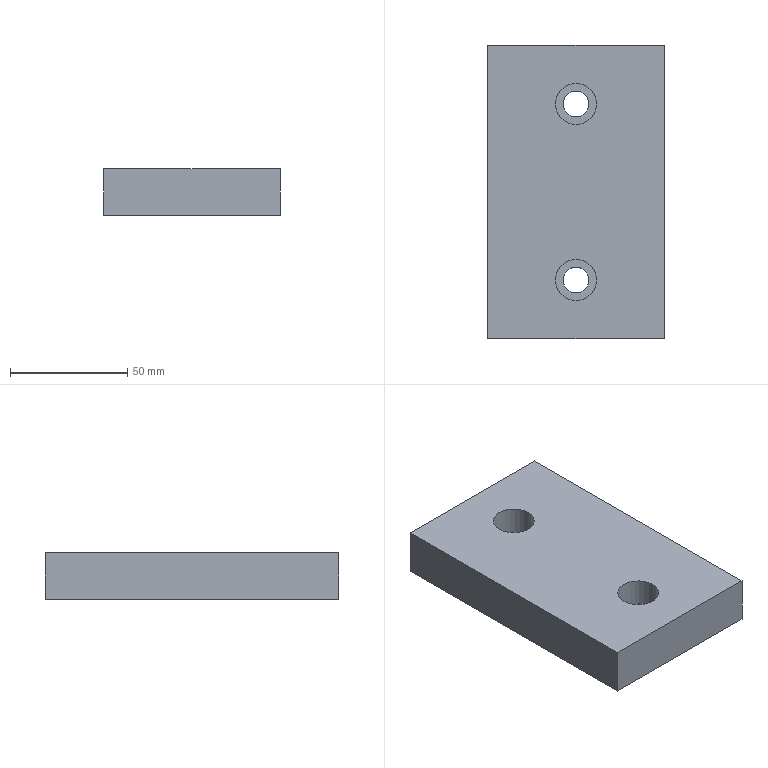Part | NX | features solid 2 | 1 solid | 12 faces | box 75 x 125 x 20 mm | volume 180207 mm3 | plane 8 | cylinder 4 | commonest cylinder face diameters 11 x2 17.5 x2
STEP:
#1=CARTESIAN_POINT('',(741.25,395.,-470.));
#2=VERTEX_POINT('',#1);
#3=CARTESIAN_POINT('',(732.5,395.,-470.));
#4=DIRECTION('',(0.,0.,1.));
#5=DIRECTION('',(1.,0.,0.));
#6=AXIS2_PLACEMENT_3D('',#3,#4,#5);
#7=CIRCLE('',#6,8.75);
#8=EDGE_CURVE('',#2,#2,#7,.F.);
#9=ORIENTED_EDGE('',*,*,#8,.T.);
#10=EDGE_LOOP('',(#9));
#11=FACE_BOUND('',#10,.T.);
#12=CARTESIAN_POINT('',(695.,295.,-470.));
#13=VERTEX_POINT('',#12);
#14=CARTESIAN_POINT('',(695.,420.,-470.));
#15=VERTEX_POINT('',#14);
#16=CARTESIAN_POINT('',(695.,295.,-470.));
#17=DIRECTION('',(0.,1.,0.));
#18=VECTOR('',#17,1000.);
#19=LINE('',#16,#18);
#20=EDGE_CURVE('',#13,#15,#19,.T.);
#21=ORIENTED_EDGE('',*,*,#20,.F.);
#22=CARTESIAN_POINT('',(770.,295.,-470.));
#23=VERTEX_POINT('',#22);
#24=CARTESIAN_POINT('',(770.,295.,-470.));
#25=DIRECTION('',(-1.,0.,0.));
#26=VECTOR('',#25,1000.);
#27=LINE('',#24,#26);
#28=EDGE_CURVE('',#23,#13,#27,.T.);
#29=ORIENTED_EDGE('',*,*,#28,.F.);
#30=CARTESIAN_POINT('',(770.,420.,-470.));
#31=VERTEX_POINT('',#30);
#32=CARTESIAN_POINT('',(770.,295.,-470.));
#33=DIRECTION('',(0.,1.,0.));
#34=VECTOR('',#33,1000.);
#35=LINE('',#32,#34);
#36=EDGE_CURVE('',#23,#31,#35,.T.);
#37=ORIENTED_EDGE('',*,*,#36,.T.);
#38=CARTESIAN_POINT('',(770.,420.,-470.));
#39=DIRECTION('',(-1.,0.,0.));
#40=VECTOR('',#39,1000.);
#41=LINE('',#38,#40);
#42=EDGE_CURVE('',#31,#15,#41,.T.);
#43=ORIENTED_EDGE('',*,*,#42,.T.);
#44=EDGE_LOOP('',(#21,#29,#37,#43));
#45=FACE_BOUND('',#44,.T.);
#46=CARTESIAN_POINT('',(741.25,320.,-470.));
#47=VERTEX_POINT('',#46);
#48=CARTESIAN_POINT('',(732.5,320.,-470.));
#49=DIRECTION('',(0.,0.,1.));
#50=DIRECTION('',(1.,0.,0.));
#51=AXIS2_PLACEMENT_3D('',#48,#49,#50);
#52=CIRCLE('',#51,8.75);
#53=EDGE_CURVE('',#47,#47,#52,.F.);
#54=ORIENTED_EDGE('',*,*,#53,.T.);
#55=EDGE_LOOP('',(#54));
#56=FACE_BOUND('',#55,.T.);
#57=CARTESIAN_POINT('',(495.,445.,-470.));
#58=DIRECTION('',(0.,0.,1.));
#59=DIRECTION('',(-1.,0.,0.));
#60=AXIS2_PLACEMENT_3D('',#57,#58,#59);
#61=PLANE('',#60);
#62=ADVANCED_FACE('',(#11,#45,#56),#61,.T.);
#63=CARTESIAN_POINT('',(695.,420.,-490.));
#64=VERTEX_POINT('',#63);
#65=CARTESIAN_POINT('',(695.,420.,-490.));
#66=DIRECTION('',(0.,0.,1.));
#67=VECTOR('',#66,1000.);
#68=LINE('',#65,#67);
#69=EDGE_CURVE('',#64,#15,#68,.T.);
#70=ORIENTED_EDGE('',*,*,#69,.T.);
#71=ORIENTED_EDGE('',*,*,#42,.F.);
#72=CARTESIAN_POINT('',(770.,420.,-490.));
#73=VERTEX_POINT('',#72);
#74=CARTESIAN_POINT('',(770.,420.,-490.));
#75=DIRECTION('',(0.,0.,1.));
#76=VECTOR('',#75,1000.);
#77=LINE('',#74,#76);
#78=EDGE_CURVE('',#73,#31,#77,.T.);
#79=ORIENTED_EDGE('',*,*,#78,.F.);
#80=CARTESIAN_POINT('',(495.,420.,-490.));
#81=DIRECTION('',(1.,0.,0.));
#82=VECTOR('',#81,1000.);
#83=LINE('',#80,#82);
#84=EDGE_CURVE('',#73,#64,#83,.F.);
#85=ORIENTED_EDGE('',*,*,#84,.T.);
#86=EDGE_LOOP('',(#70,#71,#79,#85));
#87=FACE_BOUND('',#86,.T.);
#88=CARTESIAN_POINT('',(770.,420.,-490.));
#89=DIRECTION('',(0.,-1.,0.));
#90=DIRECTION('',(0.,0.,-1.));
#91=AXIS2_PLACEMENT_3D('',#88,#89,#90);
#92=PLANE('',#91);
#93=ADVANCED_FACE('',(#87),#92,.F.);
#94=CARTESIAN_POINT('',(695.,295.,-490.));
#95=VERTEX_POINT('',#94);
#96=CARTESIAN_POINT('',(695.,295.,-490.));
#97=DIRECTION('',(0.,0.,1.));
#98=VECTOR('',#97,1000.);
#99=LINE('',#96,#98);
#100=EDGE_CURVE('',#95,#13,#99,.T.);
#101=ORIENTED_EDGE('',*,*,#100,.F.);
#102=CARTESIAN_POINT('',(770.,295.,-490.));
#103=VERTEX_POINT('',#102);
#104=CARTESIAN_POINT('',(495.,295.,-490.));
#105=DIRECTION('',(1.,0.,0.));
#106=VECTOR('',#105,1000.);
#107=LINE('',#104,#106);
#108=EDGE_CURVE('',#103,#95,#107,.F.);
#109=ORIENTED_EDGE('',*,*,#108,.F.);
#110=CARTESIAN_POINT('',(770.,295.,-490.));
#111=DIRECTION('',(0.,0.,1.));
#112=VECTOR('',#111,1000.);
#113=LINE('',#110,#112);
#114=EDGE_CURVE('',#103,#23,#113,.T.);
#115=ORIENTED_EDGE('',*,*,#114,.T.);
#116=ORIENTED_EDGE('',*,*,#28,.T.);
#117=EDGE_LOOP('',(#101,#109,#115,#116));
#118=FACE_BOUND('',#117,.T.);
#119=CARTESIAN_POINT('',(770.,295.,-490.));
#120=DIRECTION('',(0.,-1.,0.));
#121=DIRECTION('',(0.,0.,-1.));
#122=AXIS2_PLACEMENT_3D('',#119,#120,#121);
#123=PLANE('',#122);
#124=ADVANCED_FACE('',(#118),#123,.T.);
#125=CARTESIAN_POINT('',(738.,320.,-490.));
#126=VERTEX_POINT('',#125);
#127=CARTESIAN_POINT('',(732.5,320.,-490.));
#128=DIRECTION('',(0.,0.,1.));
#129=DIRECTION('',(1.,0.,0.));
#130=AXIS2_PLACEMENT_3D('',#127,#128,#129);
#131=CIRCLE('',#130,5.5);
#132=EDGE_CURVE('',#126,#126,#131,.F.);
#133=ORIENTED_EDGE('',*,*,#132,.F.);
#134=EDGE_LOOP('',(#133));
#135=FACE_BOUND('',#134,.T.);
#136=CARTESIAN_POINT('',(738.,395.,-490.));
#137=VERTEX_POINT('',#136);
#138=CARTESIAN_POINT('',(732.5,395.,-490.));
#139=DIRECTION('',(0.,0.,1.));
#140=DIRECTION('',(1.,0.,0.));
#141=AXIS2_PLACEMENT_3D('',#138,#139,#140);
#142=CIRCLE('',#141,5.5);
#143=EDGE_CURVE('',#137,#137,#142,.F.);
#144=ORIENTED_EDGE('',*,*,#143,.F.);
#145=EDGE_LOOP('',(#144));
#146=FACE_BOUND('',#145,.T.);
#147=CARTESIAN_POINT('',(695.,295.,-490.));
#148=DIRECTION('',(0.,1.,0.));
#149=VECTOR('',#148,1000.);
#150=LINE('',#147,#149);
#151=EDGE_CURVE('',#64,#95,#150,.F.);
#152=ORIENTED_EDGE('',*,*,#151,.F.);
#153=ORIENTED_EDGE('',*,*,#84,.F.);
#154=CARTESIAN_POINT('',(770.,295.,-490.));
#155=DIRECTION('',(0.,1.,0.));
#156=VECTOR('',#155,1000.);
#157=LINE('',#154,#156);
#158=EDGE_CURVE('',#73,#103,#157,.F.);
#159=ORIENTED_EDGE('',*,*,#158,.T.);
#160=ORIENTED_EDGE('',*,*,#108,.T.);
#161=EDGE_LOOP('',(#152,#153,#159,#160));
#162=FACE_BOUND('',#161,.T.);
#163=CARTESIAN_POINT('',(495.,445.,-490.));
#164=DIRECTION('',(0.,0.,1.));
#165=DIRECTION('',(-1.,0.,0.));
#166=AXIS2_PLACEMENT_3D('',#163,#164,#165);
#167=PLANE('',#166);
#168=ADVANCED_FACE('',(#135,#146,#162),#167,.F.);
#169=ORIENTED_EDGE('',*,*,#78,.T.);
#170=ORIENTED_EDGE('',*,*,#36,.F.);
#171=ORIENTED_EDGE('',*,*,#114,.F.);
#172=ORIENTED_EDGE('',*,*,#158,.F.);
#173=EDGE_LOOP('',(#169,#170,#171,#172));
#174=FACE_BOUND('',#173,.T.);
#175=CARTESIAN_POINT('',(770.,295.,-490.));
#176=DIRECTION('',(-1.,0.,0.));
#177=DIRECTION('',(0.,0.,-1.));
#178=AXIS2_PLACEMENT_3D('',#175,#176,#177);
#179=PLANE('',#178);
#180=ADVANCED_FACE('',(#174),#179,.F.);
#181=ORIENTED_EDGE('',*,*,#69,.F.);
#182=ORIENTED_EDGE('',*,*,#151,.T.);
#183=ORIENTED_EDGE('',*,*,#100,.T.);
#184=ORIENTED_EDGE('',*,*,#20,.T.);
#185=EDGE_LOOP('',(#181,#182,#183,#184));
#186=FACE_BOUND('',#185,.T.);
#187=CARTESIAN_POINT('',(695.,295.,-490.));
#188=DIRECTION('',(-1.,0.,0.));
#189=DIRECTION('',(0.,0.,-1.));
#190=AXIS2_PLACEMENT_3D('',#187,#188,#189);
#191=PLANE('',#190);
#192=ADVANCED_FACE('',(#186),#191,.T.);
#193=ORIENTED_EDGE('',*,*,#143,.T.);
#194=EDGE_LOOP('',(#193));
#195=FACE_BOUND('',#194,.T.);
#196=CARTESIAN_POINT('',(738.,395.,-482.));
#197=VERTEX_POINT('',#196);
#198=CARTESIAN_POINT('',(732.5,395.,-482.));
#199=DIRECTION('',(0.,0.,1.));
#200=DIRECTION('',(1.,0.,0.));
#201=AXIS2_PLACEMENT_3D('',#198,#199,#200);
#202=CIRCLE('',#201,5.5);
#203=EDGE_CURVE('',#197,#197,#202,.T.);
#204=ORIENTED_EDGE('',*,*,#203,.T.);
#205=EDGE_LOOP('',(#204));
#206=FACE_BOUND('',#205,.T.);
#207=CARTESIAN_POINT('',(732.5,395.,-532.));
#208=DIRECTION('',(0.,0.,1.));
#209=DIRECTION('',(1.,0.,0.));
#210=AXIS2_PLACEMENT_3D('',#207,#208,#209);
#211=CYLINDRICAL_SURFACE('',#210,5.5);
#212=ADVANCED_FACE('',(#195,#206),#211,.F.);
#213=ORIENTED_EDGE('',*,*,#8,.F.);
#214=EDGE_LOOP('',(#213));
#215=FACE_BOUND('',#214,.T.);
#216=CARTESIAN_POINT('',(741.25,395.,-482.));
#217=VERTEX_POINT('',#216);
#218=CARTESIAN_POINT('',(732.5,395.,-482.));
#219=DIRECTION('',(0.,0.,1.));
#220=DIRECTION('',(1.,0.,0.));
#221=AXIS2_PLACEMENT_3D('',#218,#219,#220);
#222=CIRCLE('',#221,8.75);
#223=EDGE_CURVE('',#217,#217,#222,.T.);
#224=ORIENTED_EDGE('',*,*,#223,.F.);
#225=EDGE_LOOP('',(#224));
#226=FACE_BOUND('',#225,.T.);
#227=CARTESIAN_POINT('',(732.5,395.,-382.));
#228=DIRECTION('',(0.,0.,-1.));
#229=DIRECTION('',(-1.,0.,0.));
#230=AXIS2_PLACEMENT_3D('',#227,#228,#229);
#231=CYLINDRICAL_SURFACE('',#230,8.75);
#232=ADVANCED_FACE('',(#215,#226),#231,.F.);
#233=ORIENTED_EDGE('',*,*,#203,.F.);
#234=EDGE_LOOP('',(#233));
#235=FACE_BOUND('',#234,.T.);
#236=ORIENTED_EDGE('',*,*,#223,.T.);
#237=EDGE_LOOP('',(#236));
#238=FACE_BOUND('',#237,.T.);
#239=CARTESIAN_POINT('',(732.5,395.,-482.));
#240=DIRECTION('',(0.,0.,1.));
#241=DIRECTION('',(1.,0.,0.));
#242=AXIS2_PLACEMENT_3D('',#239,#240,#241);
#243=PLANE('',#242);
#244=ADVANCED_FACE('',(#235,#238),#243,.T.);
#245=ORIENTED_EDGE('',*,*,#132,.T.);
#246=EDGE_LOOP('',(#245));
#247=FACE_BOUND('',#246,.T.);
#248=CARTESIAN_POINT('',(738.,320.,-482.));
#249=VERTEX_POINT('',#248);
#250=CARTESIAN_POINT('',(732.5,320.,-482.));
#251=DIRECTION('',(0.,0.,1.));
#252=DIRECTION('',(1.,0.,0.));
#253=AXIS2_PLACEMENT_3D('',#250,#251,#252);
#254=CIRCLE('',#253,5.5);
#255=EDGE_CURVE('',#249,#249,#254,.T.);
#256=ORIENTED_EDGE('',*,*,#255,.T.);
#257=EDGE_LOOP('',(#256));
#258=FACE_BOUND('',#257,.T.);
#259=CARTESIAN_POINT('',(732.5,320.,-532.));
#260=DIRECTION('',(0.,0.,1.));
#261=DIRECTION('',(1.,0.,0.));
#262=AXIS2_PLACEMENT_3D('',#259,#260,#261);
#263=CYLINDRICAL_SURFACE('',#262,5.5);
#264=ADVANCED_FACE('',(#247,#258),#263,.F.);
#265=ORIENTED_EDGE('',*,*,#53,.F.);
#266=EDGE_LOOP('',(#265));
#267=FACE_BOUND('',#266,.T.);
#268=CARTESIAN_POINT('',(741.25,320.,-482.));
#269=VERTEX_POINT('',#268);
#270=CARTESIAN_POINT('',(732.5,320.,-482.));
#271=DIRECTION('',(0.,0.,1.));
#272=DIRECTION('',(1.,0.,0.));
#273=AXIS2_PLACEMENT_3D('',#270,#271,#272);
#274=CIRCLE('',#273,8.75);
#275=EDGE_CURVE('',#269,#269,#274,.T.);
#276=ORIENTED_EDGE('',*,*,#275,.F.);
#277=EDGE_LOOP('',(#276));
#278=FACE_BOUND('',#277,.T.);
#279=CARTESIAN_POINT('',(732.5,320.,-382.));
#280=DIRECTION('',(0.,0.,-1.));
#281=DIRECTION('',(-1.,0.,0.));
#282=AXIS2_PLACEMENT_3D('',#279,#280,#281);
#283=CYLINDRICAL_SURFACE('',#282,8.75);
#284=ADVANCED_FACE('',(#267,#278),#283,.F.);
#285=ORIENTED_EDGE('',*,*,#255,.F.);
#286=EDGE_LOOP('',(#285));
#287=FACE_BOUND('',#286,.T.);
#288=ORIENTED_EDGE('',*,*,#275,.T.);
#289=EDGE_LOOP('',(#288));
#290=FACE_BOUND('',#289,.T.);
#291=CARTESIAN_POINT('',(732.5,320.,-482.));
#292=DIRECTION('',(0.,0.,1.));
#293=DIRECTION('',(1.,0.,0.));
#294=AXIS2_PLACEMENT_3D('',#291,#292,#293);
#295=PLANE('',#294);
#296=ADVANCED_FACE('',(#287,#290),#295,.T.);
#297=CLOSED_SHELL('',(#62,#93,#124,#168,#180,#192,#212,#232,#244,#264,#284,#296));
#298=MANIFOLD_SOLID_BREP('',#297);
#299=(LENGTH_UNIT()NAMED_UNIT(*)SI_UNIT(.MILLI.,.METRE.));
#300=UNCERTAINTY_MEASURE_WITH_UNIT(LENGTH_MEASURE(0.00001),#299,'','');
#301=(NAMED_UNIT(*)PLANE_ANGLE_UNIT()SI_UNIT($,.RADIAN.));
#302=(NAMED_UNIT(*)SI_UNIT($,.STERADIAN.)SOLID_ANGLE_UNIT());
#303=(GEOMETRIC_REPRESENTATION_CONTEXT(3)GLOBAL_UNCERTAINTY_ASSIGNED_CONTEXT((#300))GLOBAL_UNIT_ASSIGNED_CONTEXT((#299,#301,#302))REPRESENTATION_CONTEXT('',''));
#304=ADVANCED_BREP_SHAPE_REPRESENTATION('',(#298),#303);